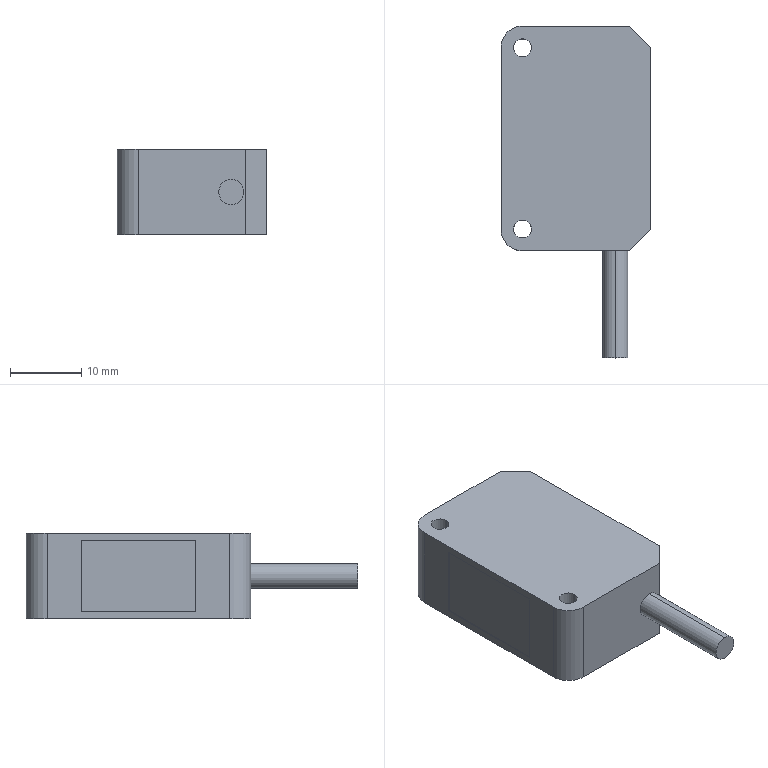Part | STEP file | BGS photoelectric switch PG6 V1.201001 | 1 solid | 22 faces | box 21 x 46.5 x 12 mm | volume 7794 mm3 | plane 14 | cylinder 8 | commonest cylinder face diameters 2.5 x4 3.5 x2 6 x2